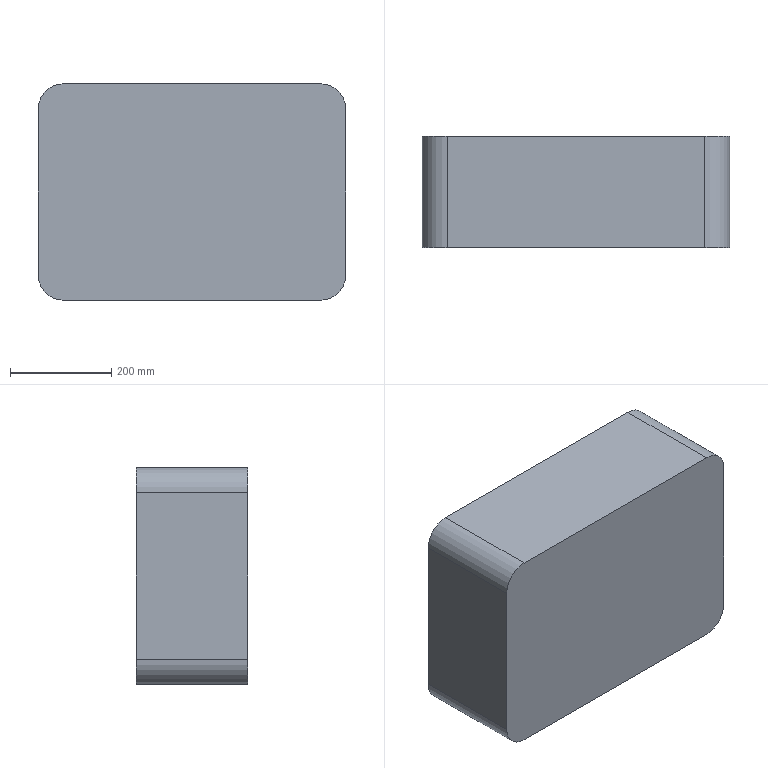Part | SolidWorks | features BaseBody 1 | 1 solid | 10 faces | box 608 x 220 x 428 mm | volume 56795852 mm3 | plane 6 | cylinder 4 | commonest cylinder face diameters 98 x4
STEP:
#1=CARTESIAN_POINT('',(255.,5.,214.));
#2=VERTEX_POINT('',#1);
#3=CARTESIAN_POINT('',(304.,5.,165.));
#4=VERTEX_POINT('',#3);
#5=CARTESIAN_POINT('',(255.,5.,165.));
#6=DIRECTION('',(0.,1.,0.));
#7=DIRECTION('',(0.,0.,1.));
#8=AXIS2_PLACEMENT_3D('',#5,#6,#7);
#9=CIRCLE('',#8,49.);
#10=EDGE_CURVE('',#2,#4,#9,.T.);
#11=ORIENTED_EDGE('',*,*,#10,.F.);
#12=CARTESIAN_POINT('',(-255.,5.,214.));
#13=VERTEX_POINT('',#12);
#14=CARTESIAN_POINT('',(-255.,5.,214.));
#15=DIRECTION('',(1.,0.,0.));
#16=VECTOR('',#15,1000.);
#17=LINE('',#14,#16);
#18=EDGE_CURVE('',#13,#2,#17,.T.);
#19=ORIENTED_EDGE('',*,*,#18,.F.);
#20=CARTESIAN_POINT('',(-304.,5.,165.));
#21=VERTEX_POINT('',#20);
#22=CARTESIAN_POINT('',(-255.,5.,165.));
#23=DIRECTION('',(0.,1.,0.));
#24=DIRECTION('',(-1.,0.,0.));
#25=AXIS2_PLACEMENT_3D('',#22,#23,#24);
#26=CIRCLE('',#25,49.);
#27=EDGE_CURVE('',#21,#13,#26,.T.);
#28=ORIENTED_EDGE('',*,*,#27,.F.);
#29=CARTESIAN_POINT('',(-304.,5.,-165.));
#30=VERTEX_POINT('',#29);
#31=CARTESIAN_POINT('',(-304.,5.,-165.));
#32=DIRECTION('',(0.,0.,1.));
#33=VECTOR('',#32,1000.);
#34=LINE('',#31,#33);
#35=EDGE_CURVE('',#30,#21,#34,.T.);
#36=ORIENTED_EDGE('',*,*,#35,.F.);
#37=CARTESIAN_POINT('',(-255.,5.,-214.));
#38=VERTEX_POINT('',#37);
#39=CARTESIAN_POINT('',(-255.,5.,-165.));
#40=DIRECTION('',(0.,1.,0.));
#41=DIRECTION('',(0.,0.,-1.));
#42=AXIS2_PLACEMENT_3D('',#39,#40,#41);
#43=CIRCLE('',#42,49.);
#44=EDGE_CURVE('',#38,#30,#43,.T.);
#45=ORIENTED_EDGE('',*,*,#44,.F.);
#46=CARTESIAN_POINT('',(255.,5.,-214.));
#47=VERTEX_POINT('',#46);
#48=CARTESIAN_POINT('',(255.,5.,-214.));
#49=DIRECTION('',(-1.,0.,0.));
#50=VECTOR('',#49,1000.);
#51=LINE('',#48,#50);
#52=EDGE_CURVE('',#47,#38,#51,.T.);
#53=ORIENTED_EDGE('',*,*,#52,.F.);
#54=CARTESIAN_POINT('',(304.,5.,-165.));
#55=VERTEX_POINT('',#54);
#56=CARTESIAN_POINT('',(255.,5.,-165.));
#57=DIRECTION('',(0.,1.,0.));
#58=DIRECTION('',(1.,0.,0.));
#59=AXIS2_PLACEMENT_3D('',#56,#57,#58);
#60=CIRCLE('',#59,49.);
#61=EDGE_CURVE('',#55,#47,#60,.T.);
#62=ORIENTED_EDGE('',*,*,#61,.F.);
#63=CARTESIAN_POINT('',(304.,5.,165.));
#64=DIRECTION('',(0.,0.,-1.));
#65=VECTOR('',#64,1000.);
#66=LINE('',#63,#65);
#67=EDGE_CURVE('',#4,#55,#66,.T.);
#68=ORIENTED_EDGE('',*,*,#67,.F.);
#69=EDGE_LOOP('',(#11,#19,#28,#36,#45,#53,#62,#68));
#70=FACE_OUTER_BOUND('',#69,.T.);
#71=CARTESIAN_POINT('',(0.,5.,0.));
#72=DIRECTION('',(0.,-1.,0.));
#73=DIRECTION('',(0.,0.,-1.));
#74=AXIS2_PLACEMENT_3D('',#71,#72,#73);
#75=PLANE('',#74);
#76=ADVANCED_FACE('',(#70),#75,.T.);
#77=CARTESIAN_POINT('',(304.,225.,165.));
#78=VERTEX_POINT('',#77);
#79=CARTESIAN_POINT('',(255.,225.,214.));
#80=VERTEX_POINT('',#79);
#81=CARTESIAN_POINT('',(255.,225.,165.));
#82=DIRECTION('',(0.,-1.,0.));
#83=DIRECTION('',(1.,0.,0.));
#84=AXIS2_PLACEMENT_3D('',#81,#82,#83);
#85=CIRCLE('',#84,49.);
#86=EDGE_CURVE('',#78,#80,#85,.T.);
#87=ORIENTED_EDGE('',*,*,#86,.F.);
#88=CARTESIAN_POINT('',(304.,225.,-165.));
#89=VERTEX_POINT('',#88);
#90=CARTESIAN_POINT('',(304.,225.,-165.));
#91=DIRECTION('',(0.,0.,1.));
#92=VECTOR('',#91,1000.);
#93=LINE('',#90,#92);
#94=EDGE_CURVE('',#89,#78,#93,.T.);
#95=ORIENTED_EDGE('',*,*,#94,.F.);
#96=CARTESIAN_POINT('',(255.,225.,-214.));
#97=VERTEX_POINT('',#96);
#98=CARTESIAN_POINT('',(255.,225.,-165.));
#99=DIRECTION('',(0.,-1.,0.));
#100=DIRECTION('',(0.,0.,-1.));
#101=AXIS2_PLACEMENT_3D('',#98,#99,#100);
#102=CIRCLE('',#101,49.);
#103=EDGE_CURVE('',#97,#89,#102,.T.);
#104=ORIENTED_EDGE('',*,*,#103,.F.);
#105=CARTESIAN_POINT('',(-255.,225.,-214.));
#106=VERTEX_POINT('',#105);
#107=CARTESIAN_POINT('',(-255.,225.,-214.));
#108=DIRECTION('',(1.,0.,0.));
#109=VECTOR('',#108,1000.);
#110=LINE('',#107,#109);
#111=EDGE_CURVE('',#106,#97,#110,.T.);
#112=ORIENTED_EDGE('',*,*,#111,.F.);
#113=CARTESIAN_POINT('',(-304.,225.,-165.));
#114=VERTEX_POINT('',#113);
#115=CARTESIAN_POINT('',(-255.,225.,-165.));
#116=DIRECTION('',(0.,-1.,0.));
#117=DIRECTION('',(-1.,0.,0.));
#118=AXIS2_PLACEMENT_3D('',#115,#116,#117);
#119=CIRCLE('',#118,49.);
#120=EDGE_CURVE('',#114,#106,#119,.T.);
#121=ORIENTED_EDGE('',*,*,#120,.F.);
#122=CARTESIAN_POINT('',(-304.,225.,165.));
#123=VERTEX_POINT('',#122);
#124=CARTESIAN_POINT('',(-304.,225.,165.));
#125=DIRECTION('',(0.,0.,-1.));
#126=VECTOR('',#125,1000.);
#127=LINE('',#124,#126);
#128=EDGE_CURVE('',#123,#114,#127,.T.);
#129=ORIENTED_EDGE('',*,*,#128,.F.);
#130=CARTESIAN_POINT('',(-255.,225.,214.));
#131=VERTEX_POINT('',#130);
#132=CARTESIAN_POINT('',(-255.,225.,165.));
#133=DIRECTION('',(0.,-1.,0.));
#134=DIRECTION('',(0.,0.,1.));
#135=AXIS2_PLACEMENT_3D('',#132,#133,#134);
#136=CIRCLE('',#135,49.);
#137=EDGE_CURVE('',#131,#123,#136,.T.);
#138=ORIENTED_EDGE('',*,*,#137,.F.);
#139=CARTESIAN_POINT('',(255.,225.,214.));
#140=DIRECTION('',(-1.,0.,0.));
#141=VECTOR('',#140,1000.);
#142=LINE('',#139,#141);
#143=EDGE_CURVE('',#80,#131,#142,.T.);
#144=ORIENTED_EDGE('',*,*,#143,.F.);
#145=EDGE_LOOP('',(#87,#95,#104,#112,#121,#129,#138,#144));
#146=FACE_OUTER_BOUND('',#145,.T.);
#147=CARTESIAN_POINT('',(0.,225.,0.));
#148=DIRECTION('',(0.,1.,0.));
#149=DIRECTION('',(1.,0.,0.));
#150=AXIS2_PLACEMENT_3D('',#147,#148,#149);
#151=PLANE('',#150);
#152=ADVANCED_FACE('',(#146),#151,.T.);
#153=ORIENTED_EDGE('',*,*,#10,.T.);
#154=CARTESIAN_POINT('',(304.,225.,165.));
#155=DIRECTION('',(0.,-1.,0.));
#156=VECTOR('',#155,1000.);
#157=LINE('',#154,#156);
#158=EDGE_CURVE('',#78,#4,#157,.T.);
#159=ORIENTED_EDGE('',*,*,#158,.F.);
#160=ORIENTED_EDGE('',*,*,#86,.T.);
#161=CARTESIAN_POINT('',(255.,5.,214.));
#162=DIRECTION('',(0.,1.,0.));
#163=VECTOR('',#162,1000.);
#164=LINE('',#161,#163);
#165=EDGE_CURVE('',#2,#80,#164,.T.);
#166=ORIENTED_EDGE('',*,*,#165,.F.);
#167=EDGE_LOOP('',(#153,#159,#160,#166));
#168=FACE_OUTER_BOUND('',#167,.T.);
#169=CARTESIAN_POINT('',(255.,5.,165.));
#170=DIRECTION('',(0.,1.,0.));
#171=DIRECTION('',(1.,0.,0.));
#172=AXIS2_PLACEMENT_3D('',#169,#170,#171);
#173=CYLINDRICAL_SURFACE('',#172,49.);
#174=ADVANCED_FACE('',(#168),#173,.T.);
#175=ORIENTED_EDGE('',*,*,#67,.T.);
#176=CARTESIAN_POINT('',(304.,225.,-165.));
#177=DIRECTION('',(0.,-1.,0.));
#178=VECTOR('',#177,1000.);
#179=LINE('',#176,#178);
#180=EDGE_CURVE('',#89,#55,#179,.T.);
#181=ORIENTED_EDGE('',*,*,#180,.F.);
#182=ORIENTED_EDGE('',*,*,#94,.T.);
#183=ORIENTED_EDGE('',*,*,#158,.T.);
#184=EDGE_LOOP('',(#175,#181,#182,#183));
#185=FACE_OUTER_BOUND('',#184,.T.);
#186=CARTESIAN_POINT('',(304.,5.,165.));
#187=DIRECTION('',(1.,0.,0.));
#188=DIRECTION('',(0.,0.,-1.));
#189=AXIS2_PLACEMENT_3D('',#186,#187,#188);
#190=PLANE('',#189);
#191=ADVANCED_FACE('',(#185),#190,.T.);
#192=ORIENTED_EDGE('',*,*,#61,.T.);
#193=CARTESIAN_POINT('',(255.,225.,-214.));
#194=DIRECTION('',(0.,-1.,0.));
#195=VECTOR('',#194,1000.);
#196=LINE('',#193,#195);
#197=EDGE_CURVE('',#97,#47,#196,.T.);
#198=ORIENTED_EDGE('',*,*,#197,.F.);
#199=ORIENTED_EDGE('',*,*,#103,.T.);
#200=ORIENTED_EDGE('',*,*,#180,.T.);
#201=EDGE_LOOP('',(#192,#198,#199,#200));
#202=FACE_OUTER_BOUND('',#201,.T.);
#203=CARTESIAN_POINT('',(255.,5.,-165.));
#204=DIRECTION('',(0.,1.,0.));
#205=DIRECTION('',(0.,0.,-1.));
#206=AXIS2_PLACEMENT_3D('',#203,#204,#205);
#207=CYLINDRICAL_SURFACE('',#206,49.);
#208=ADVANCED_FACE('',(#202),#207,.T.);
#209=ORIENTED_EDGE('',*,*,#52,.T.);
#210=CARTESIAN_POINT('',(-255.,225.,-214.));
#211=DIRECTION('',(0.,-1.,0.));
#212=VECTOR('',#211,1000.);
#213=LINE('',#210,#212);
#214=EDGE_CURVE('',#106,#38,#213,.T.);
#215=ORIENTED_EDGE('',*,*,#214,.F.);
#216=ORIENTED_EDGE('',*,*,#111,.T.);
#217=ORIENTED_EDGE('',*,*,#197,.T.);
#218=EDGE_LOOP('',(#209,#215,#216,#217));
#219=FACE_OUTER_BOUND('',#218,.T.);
#220=CARTESIAN_POINT('',(255.,5.,-214.));
#221=DIRECTION('',(0.,0.,-1.));
#222=DIRECTION('',(-1.,0.,0.));
#223=AXIS2_PLACEMENT_3D('',#220,#221,#222);
#224=PLANE('',#223);
#225=ADVANCED_FACE('',(#219),#224,.T.);
#226=ORIENTED_EDGE('',*,*,#44,.T.);
#227=CARTESIAN_POINT('',(-304.,225.,-165.));
#228=DIRECTION('',(0.,-1.,0.));
#229=VECTOR('',#228,1000.);
#230=LINE('',#227,#229);
#231=EDGE_CURVE('',#114,#30,#230,.T.);
#232=ORIENTED_EDGE('',*,*,#231,.F.);
#233=ORIENTED_EDGE('',*,*,#120,.T.);
#234=ORIENTED_EDGE('',*,*,#214,.T.);
#235=EDGE_LOOP('',(#226,#232,#233,#234));
#236=FACE_OUTER_BOUND('',#235,.T.);
#237=CARTESIAN_POINT('',(-255.,5.,-165.));
#238=DIRECTION('',(0.,1.,0.));
#239=DIRECTION('',(-1.,0.,0.));
#240=AXIS2_PLACEMENT_3D('',#237,#238,#239);
#241=CYLINDRICAL_SURFACE('',#240,49.);
#242=ADVANCED_FACE('',(#236),#241,.T.);
#243=ORIENTED_EDGE('',*,*,#35,.T.);
#244=CARTESIAN_POINT('',(-304.,225.,165.));
#245=DIRECTION('',(0.,-1.,0.));
#246=VECTOR('',#245,1000.);
#247=LINE('',#244,#246);
#248=EDGE_CURVE('',#123,#21,#247,.T.);
#249=ORIENTED_EDGE('',*,*,#248,.F.);
#250=ORIENTED_EDGE('',*,*,#128,.T.);
#251=ORIENTED_EDGE('',*,*,#231,.T.);
#252=EDGE_LOOP('',(#243,#249,#250,#251));
#253=FACE_OUTER_BOUND('',#252,.T.);
#254=CARTESIAN_POINT('',(-304.,5.,-165.));
#255=DIRECTION('',(-1.,0.,0.));
#256=DIRECTION('',(0.,1.,0.));
#257=AXIS2_PLACEMENT_3D('',#254,#255,#256);
#258=PLANE('',#257);
#259=ADVANCED_FACE('',(#253),#258,.T.);
#260=ORIENTED_EDGE('',*,*,#27,.T.);
#261=CARTESIAN_POINT('',(-255.,225.,214.));
#262=DIRECTION('',(0.,-1.,0.));
#263=VECTOR('',#262,1000.);
#264=LINE('',#261,#263);
#265=EDGE_CURVE('',#131,#13,#264,.T.);
#266=ORIENTED_EDGE('',*,*,#265,.F.);
#267=ORIENTED_EDGE('',*,*,#137,.T.);
#268=ORIENTED_EDGE('',*,*,#248,.T.);
#269=EDGE_LOOP('',(#260,#266,#267,#268));
#270=FACE_OUTER_BOUND('',#269,.T.);
#271=CARTESIAN_POINT('',(-255.,5.,165.));
#272=DIRECTION('',(0.,1.,0.));
#273=DIRECTION('',(0.,0.,1.));
#274=AXIS2_PLACEMENT_3D('',#271,#272,#273);
#275=CYLINDRICAL_SURFACE('',#274,49.);
#276=ADVANCED_FACE('',(#270),#275,.T.);
#277=ORIENTED_EDGE('',*,*,#18,.T.);
#278=ORIENTED_EDGE('',*,*,#165,.T.);
#279=ORIENTED_EDGE('',*,*,#143,.T.);
#280=ORIENTED_EDGE('',*,*,#265,.T.);
#281=EDGE_LOOP('',(#277,#278,#279,#280));
#282=FACE_OUTER_BOUND('',#281,.T.);
#283=CARTESIAN_POINT('',(-255.,5.,214.));
#284=DIRECTION('',(0.,0.,1.));
#285=DIRECTION('',(1.,0.,0.));
#286=AXIS2_PLACEMENT_3D('',#283,#284,#285);
#287=PLANE('',#286);
#288=ADVANCED_FACE('',(#282),#287,.T.);
#289=CLOSED_SHELL('',(#76,#152,#174,#191,#208,#225,#242,#259,#276,#288));
#290=MANIFOLD_SOLID_BREP('',#289);
#291=CARTESIAN_POINT('',(0.,0.,0.));
#292=DIRECTION('',(0.,0.,1.));
#293=DIRECTION('',(1.,0.,0.));
#294=AXIS2_PLACEMENT_3D('',#291,#292,#293);
#295=(LENGTH_UNIT()NAMED_UNIT(*)SI_UNIT(.MILLI.,.METRE.));
#296=UNCERTAINTY_MEASURE_WITH_UNIT(LENGTH_MEASURE(0.00001),#295,'','');
#297=(NAMED_UNIT(*)PLANE_ANGLE_UNIT()SI_UNIT($,.RADIAN.));
#298=(NAMED_UNIT(*)SI_UNIT($,.STERADIAN.)SOLID_ANGLE_UNIT());
#299=(GEOMETRIC_REPRESENTATION_CONTEXT(3)GLOBAL_UNCERTAINTY_ASSIGNED_CONTEXT((#296))GLOBAL_UNIT_ASSIGNED_CONTEXT((#295,#297,#298))REPRESENTATION_CONTEXT('',''));
#300=ADVANCED_BREP_SHAPE_REPRESENTATION('',(#290,#294),#299);